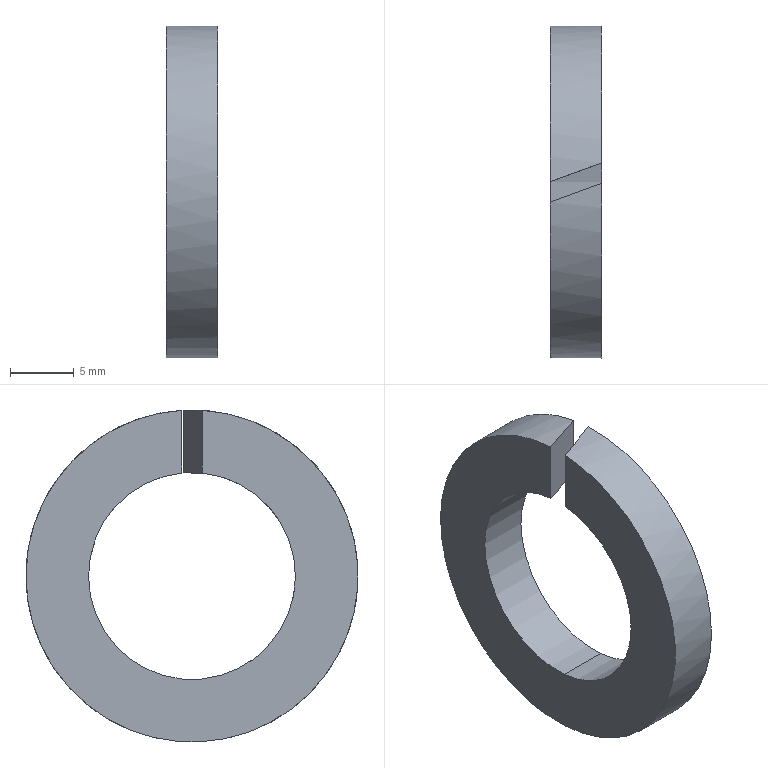Part | STEP file | KS B 1324 - No. 2 - 16 | 1 solid | 8 faces | box 4 x 26 x 26 mm | volume 1268 mm3 | cylinder 4 | plane 4 | commonest cylinder face diameters 16.2 x2 26 x2
STEP:
#1=CARTESIAN_POINT('',(0.,0.,0.));
#2=DIRECTION('',(0.,0.,1.));
#3=DIRECTION('',(1.,0.,0.));
#4=AXIS2_PLACEMENT_3D('',#1,#2,#3);
#5=CARTESIAN_POINT('',(4.,2.256,7.78));
#6=VERTEX_POINT('',#5);
#7=CARTESIAN_POINT('',(0.,0.8,8.06));
#8=VERTEX_POINT('',#7);
#9=CARTESIAN_POINT('',(4.,2.256,7.78));
#10=CARTESIAN_POINT('',(2.692,1.78,7.918));
#11=CARTESIAN_POINT('',(1.355,1.293,8.011));
#12=CARTESIAN_POINT('',(0.,0.8,8.06));
#13=(BOUNDED_CURVE()B_SPLINE_CURVE(3,(#9,#10,#11,#12),.UNSPECIFIED.,.F.,.F.)B_SPLINE_CURVE_WITH_KNOTS((4,4),(4.43,4.613),.PIECEWISE_BEZIER_KNOTS.)CURVE()GEOMETRIC_REPRESENTATION_ITEM()RATIONAL_B_SPLINE_CURVE((1.,0.9972,0.9972,1.))REPRESENTATION_ITEM(''));
#14=CARTESIAN_POINT('',(0.,0.,0.));
#15=DIRECTION('',(1.,0.,0.));
#16=DIRECTION('',(0.,-0.08987,-0.996));
#17=AXIS2_PLACEMENT_3D('',#14,#15,#16);
#18=CYLINDRICAL_SURFACE('',#17,8.1);
#19=CARTESIAN_POINT('',(2.949,4.));
#20=CARTESIAN_POINT('',(2.952,3.941));
#21=CARTESIAN_POINT('',(2.958,3.822));
#22=CARTESIAN_POINT('',(2.966,3.643));
#23=CARTESIAN_POINT('',(2.974,3.464));
#24=CARTESIAN_POINT('',(2.983,3.285));
#25=CARTESIAN_POINT('',(2.991,3.105));
#26=CARTESIAN_POINT('',(2.999,2.925));
#27=CARTESIAN_POINT('',(3.008,2.744));
#28=CARTESIAN_POINT('',(3.016,2.563));
#29=CARTESIAN_POINT('',(3.024,2.382));
#30=CARTESIAN_POINT('',(3.033,2.2));
#31=CARTESIAN_POINT('',(3.041,2.018));
#32=CARTESIAN_POINT('',(3.049,1.835));
#33=CARTESIAN_POINT('',(3.058,1.653));
#34=CARTESIAN_POINT('',(3.066,1.47));
#35=CARTESIAN_POINT('',(3.074,1.287));
#36=CARTESIAN_POINT('',(3.083,1.103));
#37=CARTESIAN_POINT('',(3.091,0.9199));
#38=CARTESIAN_POINT('',(3.099,0.7362));
#39=CARTESIAN_POINT('',(3.108,0.5524));
#40=CARTESIAN_POINT('',(3.116,0.3684));
#41=CARTESIAN_POINT('',(3.124,0.1842));
#42=CARTESIAN_POINT('',(3.13,0.06142));
#43=CARTESIAN_POINT('',(3.133,0.));
#44=B_SPLINE_CURVE_WITH_KNOTS('',3,(#19,#20,#21,#22,#23,#24,#25,#26,#27,#28,#29,#30,#31,#32,#33,#34,#35,#36,#37,#38,#39,#40,#41,#42,#43),.UNSPECIFIED.,.F.,.F.,(4,1,1,1,1,1,1,1,1,1,1,1,1,1,1,1,1,1,1,1,1,1,4),(4.43,4.438,4.447,4.455,4.463,4.472,4.48,4.488,4.497,4.505,4.513,4.522,4.53,4.538,4.547,4.555,4.563,4.572,4.58,4.588,4.597,4.605,4.613),.QUASI_UNIFORM_KNOTS.);
#45=(GEOMETRIC_REPRESENTATION_CONTEXT(2)PARAMETRIC_REPRESENTATION_CONTEXT()REPRESENTATION_CONTEXT('',''));
#46=DEFINITIONAL_REPRESENTATION('',(#44),#45);
#47=PCURVE('',#18,#46);
#48=CARTESIAN_POINT('',(0.,0.8,0.));
#49=DIRECTION('',(-0.342,0.9397,0.));
#50=DIRECTION('',(0.,0.,1.));
#51=AXIS2_PLACEMENT_3D('',#48,#49,#50);
#52=PLANE('',#51);
#53=CARTESIAN_POINT('',(7.78,4.257));
#54=CARTESIAN_POINT('',(7.918,2.865));
#55=CARTESIAN_POINT('',(8.011,1.442));
#56=CARTESIAN_POINT('',(8.06,0.));
#57=(BOUNDED_CURVE()B_SPLINE_CURVE(3,(#53,#54,#55,#56),.UNSPECIFIED.,.F.,.F.)B_SPLINE_CURVE_WITH_KNOTS((4,4),(4.43,4.613),.PIECEWISE_BEZIER_KNOTS.)CURVE()GEOMETRIC_REPRESENTATION_ITEM()RATIONAL_B_SPLINE_CURVE((1.,0.9972,0.9972,1.))REPRESENTATION_ITEM(''));
#58=(GEOMETRIC_REPRESENTATION_CONTEXT(2)PARAMETRIC_REPRESENTATION_CONTEXT()REPRESENTATION_CONTEXT('',''));
#59=DEFINITIONAL_REPRESENTATION('',(#57),#58);
#60=PCURVE('',#52,#59);
#61=SURFACE_CURVE('',#13,(#47,#60),.PCURVE_S1.);
#62=EDGE_CURVE('',#6,#8,#61,.T.);
#63=ORIENTED_EDGE('',*,*,#62,.F.);
#64=CARTESIAN_POINT('',(4.,-0.728,-8.067));
#65=VERTEX_POINT('',#64);
#66=CARTESIAN_POINT('',(4.,0.,0.));
#67=DIRECTION('',(-1.,0.,0.));
#68=DIRECTION('',(0.,-1.,0.));
#69=AXIS2_PLACEMENT_3D('',#66,#67,#68);
#70=CIRCLE('',#69,8.1);
#71=CARTESIAN_POINT('',(4.802,4.));
#72=DIRECTION('',(-1.,0.));
#73=VECTOR('',#72,1.);
#74=LINE('',#71,#73);
#75=(GEOMETRIC_REPRESENTATION_CONTEXT(2)PARAMETRIC_REPRESENTATION_CONTEXT()REPRESENTATION_CONTEXT('',''));
#76=DEFINITIONAL_REPRESENTATION('',(#74),#75);
#77=PCURVE('',#18,#76);
#78=CARTESIAN_POINT('',(4.,0.,0.));
#79=DIRECTION('',(-1.,0.,0.));
#80=DIRECTION('',(0.,0.,1.));
#81=AXIS2_PLACEMENT_3D('',#78,#79,#80);
#82=PLANE('',#81);
#83=CARTESIAN_POINT('',(0.,0.));
#84=DIRECTION('',(0.,-1.));
#85=AXIS2_PLACEMENT_2D('',#83,#84);
#86=CIRCLE('',#85,8.1);
#87=(GEOMETRIC_REPRESENTATION_CONTEXT(2)PARAMETRIC_REPRESENTATION_CONTEXT()REPRESENTATION_CONTEXT('',''));
#88=DEFINITIONAL_REPRESENTATION('',(#86),#87);
#89=PCURVE('',#82,#88);
#90=SURFACE_CURVE('',#70,(#77,#89),.PCURVE_S1.);
#91=EDGE_CURVE('',#6,#65,#90,.T.);
#92=ORIENTED_EDGE('',*,*,#91,.T.);
#93=CARTESIAN_POINT('',(0.,-0.728,-8.067));
#94=VERTEX_POINT('',#93);
#95=CARTESIAN_POINT('',(0.,-0.728,-8.067));
#96=DIRECTION('',(1.,0.,0.));
#97=VECTOR('',#96,1.);
#98=LINE('',#95,#97);
#99=CARTESIAN_POINT('',(0.,0.));
#100=DIRECTION('',(0.,1.));
#101=VECTOR('',#100,1.);
#102=LINE('',#99,#101);
#103=(GEOMETRIC_REPRESENTATION_CONTEXT(2)PARAMETRIC_REPRESENTATION_CONTEXT()REPRESENTATION_CONTEXT('',''));
#104=DEFINITIONAL_REPRESENTATION('',(#102),#103);
#105=PCURVE('',#18,#104);
#106=CARTESIAN_POINT('',(0.,0.,0.));
#107=DIRECTION('',(1.,0.,0.));
#108=DIRECTION('',(0.,-0.08987,-0.996));
#109=AXIS2_PLACEMENT_3D('',#106,#107,#108);
#110=CYLINDRICAL_SURFACE('',#109,8.1);
#111=CARTESIAN_POINT('',(6.283,0.));
#112=DIRECTION('',(0.,1.));
#113=VECTOR('',#112,1.);
#114=LINE('',#111,#113);
#115=(GEOMETRIC_REPRESENTATION_CONTEXT(2)PARAMETRIC_REPRESENTATION_CONTEXT()REPRESENTATION_CONTEXT('',''));
#116=DEFINITIONAL_REPRESENTATION('',(#114),#115);
#117=PCURVE('',#110,#116);
#118=SURFACE_CURVE('',#98,(#105,#117),.PCURVE_S1.);
#119=EDGE_CURVE('',#94,#65,#118,.T.);
#120=ORIENTED_EDGE('',*,*,#119,.F.);
#121=CARTESIAN_POINT('',(0.,0.,0.));
#122=DIRECTION('',(1.,0.,0.));
#123=DIRECTION('',(0.,-1.,0.));
#124=AXIS2_PLACEMENT_3D('',#121,#122,#123);
#125=CIRCLE('',#124,8.1);
#126=CARTESIAN_POINT('',(-1.481,0.));
#127=DIRECTION('',(1.,0.));
#128=VECTOR('',#127,1.);
#129=LINE('',#126,#128);
#130=(GEOMETRIC_REPRESENTATION_CONTEXT(2)PARAMETRIC_REPRESENTATION_CONTEXT()REPRESENTATION_CONTEXT('',''));
#131=DEFINITIONAL_REPRESENTATION('',(#129),#130);
#132=PCURVE('',#18,#131);
#133=CARTESIAN_POINT('',(0.,0.,0.));
#134=DIRECTION('',(-1.,0.,0.));
#135=DIRECTION('',(0.,0.,1.));
#136=AXIS2_PLACEMENT_3D('',#133,#134,#135);
#137=PLANE('',#136);
#138=CARTESIAN_POINT('',(0.,-8.1));
#139=CARTESIAN_POINT('',(-14.03,-8.1));
#140=CARTESIAN_POINT('',(-7.015,4.05));
#141=CARTESIAN_POINT('',(0.,16.2));
#142=CARTESIAN_POINT('',(7.015,4.05));
#143=CARTESIAN_POINT('',(14.03,-8.1));
#144=CARTESIAN_POINT('',(0.,-8.1));
#145=(BOUNDED_CURVE()B_SPLINE_CURVE(2,(#138,#139,#140,#141,#142,#143,#144),.UNSPECIFIED.,.T.,.F.)B_SPLINE_CURVE_WITH_KNOTS((1,2,2,2,2,1),(-2.094,0.,2.094,4.189,6.283,8.378),.UNSPECIFIED.)CURVE()GEOMETRIC_REPRESENTATION_ITEM()RATIONAL_B_SPLINE_CURVE((1.,0.5,1.,0.5,1.,0.5,1.))REPRESENTATION_ITEM(''));
#146=(GEOMETRIC_REPRESENTATION_CONTEXT(2)PARAMETRIC_REPRESENTATION_CONTEXT()REPRESENTATION_CONTEXT('',''));
#147=DEFINITIONAL_REPRESENTATION('',(#145),#146);
#148=PCURVE('',#137,#147);
#149=SURFACE_CURVE('',#125,(#132,#148),.PCURVE_S1.);
#150=EDGE_CURVE('',#94,#8,#149,.T.);
#151=ORIENTED_EDGE('',*,*,#150,.T.);
#152=EDGE_LOOP('',(#63,#92,#120,#151));
#153=FACE_BOUND('',#152,.F.);
#154=ADVANCED_FACE('',(#153),#18,.F.);
#155=CARTESIAN_POINT('',(0.,-0.728,-12.98));
#156=VERTEX_POINT('',#155);
#157=CARTESIAN_POINT('',(0.,-0.8,12.975));
#158=VERTEX_POINT('',#157);
#159=CARTESIAN_POINT('',(0.,0.,0.));
#160=DIRECTION('',(-1.,0.,0.));
#161=DIRECTION('',(0.,-1.,0.));
#162=AXIS2_PLACEMENT_3D('',#159,#160,#161);
#163=CIRCLE('',#162,13.);
#164=CARTESIAN_POINT('',(0.,0.,0.));
#165=DIRECTION('',(1.,0.,0.));
#166=DIRECTION('',(0.,-0.056,-0.9984));
#167=AXIS2_PLACEMENT_3D('',#164,#165,#166);
#168=CYLINDRICAL_SURFACE('',#167,13.);
#169=CARTESIAN_POINT('',(11.052,0.));
#170=DIRECTION('',(-1.,0.));
#171=VECTOR('',#170,1.);
#172=LINE('',#169,#171);
#173=(GEOMETRIC_REPRESENTATION_CONTEXT(2)PARAMETRIC_REPRESENTATION_CONTEXT()REPRESENTATION_CONTEXT('',''));
#174=DEFINITIONAL_REPRESENTATION('',(#172),#173);
#175=PCURVE('',#168,#174);
#176=CARTESIAN_POINT('',(0.,0.));
#177=DIRECTION('',(0.,-1.));
#178=AXIS2_PLACEMENT_2D('',#176,#177);
#179=CIRCLE('',#178,13.);
#180=(GEOMETRIC_REPRESENTATION_CONTEXT(2)PARAMETRIC_REPRESENTATION_CONTEXT()REPRESENTATION_CONTEXT('',''));
#181=DEFINITIONAL_REPRESENTATION('',(#179),#180);
#182=PCURVE('',#137,#181);
#183=SURFACE_CURVE('',#163,(#175,#182),.PCURVE_S1.);
#184=EDGE_CURVE('',#156,#158,#183,.T.);
#185=ORIENTED_EDGE('',*,*,#184,.F.);
#186=CARTESIAN_POINT('',(4.,-0.728,-12.98));
#187=VERTEX_POINT('',#186);
#188=CARTESIAN_POINT('',(0.,-0.728,-12.98));
#189=DIRECTION('',(1.,0.,0.));
#190=VECTOR('',#189,1.);
#191=LINE('',#188,#190);
#192=CARTESIAN_POINT('',(6.283,0.));
#193=DIRECTION('',(0.,1.));
#194=VECTOR('',#193,1.);
#195=LINE('',#192,#194);
#196=(GEOMETRIC_REPRESENTATION_CONTEXT(2)PARAMETRIC_REPRESENTATION_CONTEXT()REPRESENTATION_CONTEXT('',''));
#197=DEFINITIONAL_REPRESENTATION('',(#195),#196);
#198=PCURVE('',#168,#197);
#199=CARTESIAN_POINT('',(0.,0.,0.));
#200=DIRECTION('',(1.,0.,0.));
#201=DIRECTION('',(0.,-0.056,-0.9984));
#202=AXIS2_PLACEMENT_3D('',#199,#200,#201);
#203=CYLINDRICAL_SURFACE('',#202,13.);
#204=CARTESIAN_POINT('',(0.,0.));
#205=DIRECTION('',(0.,1.));
#206=VECTOR('',#205,1.);
#207=LINE('',#204,#206);
#208=(GEOMETRIC_REPRESENTATION_CONTEXT(2)PARAMETRIC_REPRESENTATION_CONTEXT()REPRESENTATION_CONTEXT('',''));
#209=DEFINITIONAL_REPRESENTATION('',(#207),#208);
#210=PCURVE('',#203,#209);
#211=SURFACE_CURVE('',#191,(#198,#210),.PCURVE_S1.);
#212=EDGE_CURVE('',#156,#187,#211,.T.);
#213=ORIENTED_EDGE('',*,*,#212,.T.);
#214=CARTESIAN_POINT('',(4.,0.6559,12.983));
#215=VERTEX_POINT('',#214);
#216=CARTESIAN_POINT('',(4.,0.,0.));
#217=DIRECTION('',(-1.,0.,0.));
#218=DIRECTION('',(0.,-1.,0.));
#219=AXIS2_PLACEMENT_3D('',#216,#217,#218);
#220=CIRCLE('',#219,13.);
#221=CARTESIAN_POINT('',(11.052,4.));
#222=DIRECTION('',(-1.,0.));
#223=VECTOR('',#222,1.);
#224=LINE('',#221,#223);
#225=(GEOMETRIC_REPRESENTATION_CONTEXT(2)PARAMETRIC_REPRESENTATION_CONTEXT()REPRESENTATION_CONTEXT('',''));
#226=DEFINITIONAL_REPRESENTATION('',(#224),#225);
#227=PCURVE('',#168,#226);
#228=CARTESIAN_POINT('',(0.,0.));
#229=DIRECTION('',(0.,-1.));
#230=AXIS2_PLACEMENT_2D('',#228,#229);
#231=CIRCLE('',#230,13.);
#232=(GEOMETRIC_REPRESENTATION_CONTEXT(2)PARAMETRIC_REPRESENTATION_CONTEXT()REPRESENTATION_CONTEXT('',''));
#233=DEFINITIONAL_REPRESENTATION('',(#231),#232);
#234=PCURVE('',#82,#233);
#235=SURFACE_CURVE('',#220,(#227,#234),.PCURVE_S1.);
#236=EDGE_CURVE('',#187,#215,#235,.T.);
#237=ORIENTED_EDGE('',*,*,#236,.T.);
#238=CARTESIAN_POINT('',(4.,0.6559,12.983));
#239=CARTESIAN_POINT('',(2.667,0.1707,13.008));
#240=CARTESIAN_POINT('',(1.332,-0.3151,13.005));
#241=CARTESIAN_POINT('',(0.,-0.8,12.975));
#242=(BOUNDED_CURVE()B_SPLINE_CURVE(3,(#238,#239,#240,#241),.UNSPECIFIED.,.F.,.F.)B_SPLINE_CURVE_WITH_KNOTS((4,4),(4.662,4.774),.PIECEWISE_BEZIER_KNOTS.)CURVE()GEOMETRIC_REPRESENTATION_ITEM()RATIONAL_B_SPLINE_CURVE((1.,0.999,0.999,1.))REPRESENTATION_ITEM(''));
#243=CARTESIAN_POINT('',(3.147,4.));
#244=CARTESIAN_POINT('',(3.149,3.939));
#245=CARTESIAN_POINT('',(3.152,3.818));
#246=CARTESIAN_POINT('',(3.157,3.637));
#247=CARTESIAN_POINT('',(3.162,3.455));
#248=CARTESIAN_POINT('',(3.168,3.273));
#249=CARTESIAN_POINT('',(3.173,3.091));
#250=CARTESIAN_POINT('',(3.178,2.909));
#251=CARTESIAN_POINT('',(3.183,2.728));
#252=CARTESIAN_POINT('',(3.188,2.546));
#253=CARTESIAN_POINT('',(3.193,2.364));
#254=CARTESIAN_POINT('',(3.198,2.182));
#255=CARTESIAN_POINT('',(3.203,2.));
#256=CARTESIAN_POINT('',(3.208,1.818));
#257=CARTESIAN_POINT('',(3.213,1.636));
#258=CARTESIAN_POINT('',(3.218,1.454));
#259=CARTESIAN_POINT('',(3.224,1.272));
#260=CARTESIAN_POINT('',(3.229,1.09));
#261=CARTESIAN_POINT('',(3.234,0.9083));
#262=CARTESIAN_POINT('',(3.239,0.7265));
#263=CARTESIAN_POINT('',(3.244,0.5448));
#264=CARTESIAN_POINT('',(3.249,0.3631));
#265=CARTESIAN_POINT('',(3.254,0.1815));
#266=CARTESIAN_POINT('',(3.257,0.06049));
#267=CARTESIAN_POINT('',(3.259,0.));
#268=B_SPLINE_CURVE_WITH_KNOTS('',3,(#243,#244,#245,#246,#247,#248,#249,#250,#251,#252,#253,#254,#255,#256,#257,#258,#259,#260,#261,#262,#263,#264,#265,#266,#267),.UNSPECIFIED.,.F.,.F.,(4,1,1,1,1,1,1,1,1,1,1,1,1,1,1,1,1,1,1,1,1,1,4),(4.662,4.667,4.672,4.677,4.682,4.687,4.692,4.698,4.703,4.708,4.713,4.718,4.723,4.728,4.733,4.738,4.743,4.749,4.754,4.759,4.764,4.769,4.774),.QUASI_UNIFORM_KNOTS.);
#269=(GEOMETRIC_REPRESENTATION_CONTEXT(2)PARAMETRIC_REPRESENTATION_CONTEXT()REPRESENTATION_CONTEXT('',''));
#270=DEFINITIONAL_REPRESENTATION('',(#268),#269);
#271=PCURVE('',#168,#270);
#272=CARTESIAN_POINT('',(4.,0.6559,0.));
#273=DIRECTION('',(0.342,-0.9397,0.));
#274=DIRECTION('',(0.,0.,-1.));
#275=AXIS2_PLACEMENT_3D('',#272,#273,#274);
#276=PLANE('',#275);
#277=CARTESIAN_POINT('',(-12.983,0.));
#278=CARTESIAN_POINT('',(-13.008,-1.419));
#279=CARTESIAN_POINT('',(-13.005,-2.839));
#280=CARTESIAN_POINT('',(-12.975,-4.257));
#281=(BOUNDED_CURVE()B_SPLINE_CURVE(3,(#277,#278,#279,#280),.UNSPECIFIED.,.F.,.F.)B_SPLINE_CURVE_WITH_KNOTS((4,4),(4.662,4.774),.PIECEWISE_BEZIER_KNOTS.)CURVE()GEOMETRIC_REPRESENTATION_ITEM()RATIONAL_B_SPLINE_CURVE((1.,0.999,0.999,1.))REPRESENTATION_ITEM(''));
#282=(GEOMETRIC_REPRESENTATION_CONTEXT(2)PARAMETRIC_REPRESENTATION_CONTEXT()REPRESENTATION_CONTEXT('',''));
#283=DEFINITIONAL_REPRESENTATION('',(#281),#282);
#284=PCURVE('',#276,#283);
#285=SURFACE_CURVE('',#242,(#271,#284),.PCURVE_S1.);
#286=EDGE_CURVE('',#215,#158,#285,.T.);
#287=ORIENTED_EDGE('',*,*,#286,.T.);
#288=EDGE_LOOP('',(#185,#213,#237,#287));
#289=FACE_BOUND('',#288,.T.);
#290=ADVANCED_FACE('',(#289),#168,.T.);
#291=CARTESIAN_POINT('',(0.,-0.8,8.06));
#292=VERTEX_POINT('',#291);
#293=CARTESIAN_POINT('',(0.,-0.8,0.));
#294=DIRECTION('',(0.,0.,-1.));
#295=VECTOR('',#294,1.);
#296=LINE('',#293,#295);
#297=CARTESIAN_POINT('',(0.,-0.8));
#298=DIRECTION('',(-1.,0.));
#299=VECTOR('',#298,1.);
#300=LINE('',#297,#299);
#301=(GEOMETRIC_REPRESENTATION_CONTEXT(2)PARAMETRIC_REPRESENTATION_CONTEXT()REPRESENTATION_CONTEXT('',''));
#302=DEFINITIONAL_REPRESENTATION('',(#300),#301);
#303=PCURVE('',#137,#302);
#304=CARTESIAN_POINT('',(0.,-4.257));
#305=DIRECTION('',(1.,0.));
#306=VECTOR('',#305,1.);
#307=LINE('',#304,#306);
#308=(GEOMETRIC_REPRESENTATION_CONTEXT(2)PARAMETRIC_REPRESENTATION_CONTEXT()REPRESENTATION_CONTEXT('',''));
#309=DEFINITIONAL_REPRESENTATION('',(#307),#308);
#310=PCURVE('',#276,#309);
#311=SURFACE_CURVE('',#296,(#303,#310),.PCURVE_S1.);
#312=EDGE_CURVE('',#158,#292,#311,.T.);
#313=ORIENTED_EDGE('',*,*,#312,.T.);
#314=CARTESIAN_POINT('',(0.,0.,0.));
#315=DIRECTION('',(1.,0.,0.));
#316=DIRECTION('',(0.,-1.,0.));
#317=AXIS2_PLACEMENT_3D('',#314,#315,#316);
#318=CIRCLE('',#317,8.1);
#319=CARTESIAN_POINT('',(0.,-8.1));
#320=CARTESIAN_POINT('',(-14.03,-8.1));
#321=CARTESIAN_POINT('',(-7.015,4.05));
#322=CARTESIAN_POINT('',(0.,16.2));
#323=CARTESIAN_POINT('',(7.015,4.05));
#324=CARTESIAN_POINT('',(14.03,-8.1));
#325=CARTESIAN_POINT('',(0.,-8.1));
#326=(BOUNDED_CURVE()B_SPLINE_CURVE(2,(#319,#320,#321,#322,#323,#324,#325),.UNSPECIFIED.,.T.,.F.)B_SPLINE_CURVE_WITH_KNOTS((1,2,2,2,2,1),(-2.094,0.,2.094,4.189,6.283,8.378),.UNSPECIFIED.)CURVE()GEOMETRIC_REPRESENTATION_ITEM()RATIONAL_B_SPLINE_CURVE((1.,0.5,1.,0.5,1.,0.5,1.))REPRESENTATION_ITEM(''));
#327=(GEOMETRIC_REPRESENTATION_CONTEXT(2)PARAMETRIC_REPRESENTATION_CONTEXT()REPRESENTATION_CONTEXT('',''));
#328=DEFINITIONAL_REPRESENTATION('',(#326),#327);
#329=PCURVE('',#137,#328);
#330=CARTESIAN_POINT('',(-1.481,0.));
#331=DIRECTION('',(1.,0.));
#332=VECTOR('',#331,1.);
#333=LINE('',#330,#332);
#334=(GEOMETRIC_REPRESENTATION_CONTEXT(2)PARAMETRIC_REPRESENTATION_CONTEXT()REPRESENTATION_CONTEXT('',''));
#335=DEFINITIONAL_REPRESENTATION('',(#333),#334);
#336=PCURVE('',#110,#335);
#337=SURFACE_CURVE('',#318,(#329,#336),.PCURVE_S1.);
#338=EDGE_CURVE('',#292,#94,#337,.T.);
#339=ORIENTED_EDGE('',*,*,#338,.T.);
#340=ORIENTED_EDGE('',*,*,#150,.T.);
#341=CARTESIAN_POINT('',(0.,0.8,12.975));
#342=VERTEX_POINT('',#341);
#343=CARTESIAN_POINT('',(0.,0.8,0.));
#344=DIRECTION('',(0.,0.,1.));
#345=VECTOR('',#344,1.);
#346=LINE('',#343,#345);
#347=CARTESIAN_POINT('',(0.,0.8));
#348=DIRECTION('',(1.,0.));
#349=VECTOR('',#348,1.);
#350=LINE('',#347,#349);
#351=(GEOMETRIC_REPRESENTATION_CONTEXT(2)PARAMETRIC_REPRESENTATION_CONTEXT()REPRESENTATION_CONTEXT('',''));
#352=DEFINITIONAL_REPRESENTATION('',(#350),#351);
#353=PCURVE('',#137,#352);
#354=CARTESIAN_POINT('',(0.,0.));
#355=DIRECTION('',(1.,0.));
#356=VECTOR('',#355,1.);
#357=LINE('',#354,#356);
#358=(GEOMETRIC_REPRESENTATION_CONTEXT(2)PARAMETRIC_REPRESENTATION_CONTEXT()REPRESENTATION_CONTEXT('',''));
#359=DEFINITIONAL_REPRESENTATION('',(#357),#358);
#360=PCURVE('',#52,#359);
#361=SURFACE_CURVE('',#346,(#353,#360),.PCURVE_S1.);
#362=EDGE_CURVE('',#8,#342,#361,.T.);
#363=ORIENTED_EDGE('',*,*,#362,.T.);
#364=CARTESIAN_POINT('',(0.,0.,0.));
#365=DIRECTION('',(-1.,0.,0.));
#366=DIRECTION('',(0.,-1.,0.));
#367=AXIS2_PLACEMENT_3D('',#364,#365,#366);
#368=CIRCLE('',#367,13.);
#369=CARTESIAN_POINT('',(0.,0.));
#370=DIRECTION('',(0.,-1.));
#371=AXIS2_PLACEMENT_2D('',#369,#370);
#372=CIRCLE('',#371,13.);
#373=(GEOMETRIC_REPRESENTATION_CONTEXT(2)PARAMETRIC_REPRESENTATION_CONTEXT()REPRESENTATION_CONTEXT('',''));
#374=DEFINITIONAL_REPRESENTATION('',(#372),#373);
#375=PCURVE('',#137,#374);
#376=CARTESIAN_POINT('',(4.768,0.));
#377=DIRECTION('',(-1.,0.));
#378=VECTOR('',#377,1.);
#379=LINE('',#376,#378);
#380=(GEOMETRIC_REPRESENTATION_CONTEXT(2)PARAMETRIC_REPRESENTATION_CONTEXT()REPRESENTATION_CONTEXT('',''));
#381=DEFINITIONAL_REPRESENTATION('',(#379),#380);
#382=PCURVE('',#203,#381);
#383=SURFACE_CURVE('',#368,(#375,#382),.PCURVE_S1.);
#384=EDGE_CURVE('',#342,#156,#383,.T.);
#385=ORIENTED_EDGE('',*,*,#384,.T.);
#386=ORIENTED_EDGE('',*,*,#184,.T.);
#387=EDGE_LOOP('',(#313,#339,#340,#363,#385,#386));
#388=FACE_BOUND('',#387,.T.);
#389=ADVANCED_FACE('',(#388),#137,.T.);
#390=ORIENTED_EDGE('',*,*,#212,.F.);
#391=ORIENTED_EDGE('',*,*,#384,.F.);
#392=CARTESIAN_POINT('',(4.,2.256,12.803));
#393=VERTEX_POINT('',#392);
#394=CARTESIAN_POINT('',(0.,0.8,12.975));
#395=CARTESIAN_POINT('',(1.342,1.288,12.945));
#396=CARTESIAN_POINT('',(2.676,1.774,12.888));
#397=CARTESIAN_POINT('',(4.,2.256,12.803));
#398=(BOUNDED_CURVE()B_SPLINE_CURVE(3,(#394,#395,#396,#397),.UNSPECIFIED.,.F.,.F.)B_SPLINE_CURVE_WITH_KNOTS((4,4),(1.632,1.745),.PIECEWISE_BEZIER_KNOTS.)CURVE()GEOMETRIC_REPRESENTATION_ITEM()RATIONAL_B_SPLINE_CURVE((1.,0.9989,0.9989,1.))REPRESENTATION_ITEM(''));
#399=CARTESIAN_POINT('',(3.136,0.));
#400=CARTESIAN_POINT('',(3.134,0.06091));
#401=CARTESIAN_POINT('',(3.131,0.1827));
#402=CARTESIAN_POINT('',(3.126,0.3654));
#403=CARTESIAN_POINT('',(3.121,0.5481));
#404=CARTESIAN_POINT('',(3.116,0.7307));
#405=CARTESIAN_POINT('',(3.11,0.9132));
#406=CARTESIAN_POINT('',(3.105,1.096));
#407=CARTESIAN_POINT('',(3.1,1.278));
#408=CARTESIAN_POINT('',(3.095,1.46));
#409=CARTESIAN_POINT('',(3.09,1.643));
#410=CARTESIAN_POINT('',(3.085,1.825));
#411=CARTESIAN_POINT('',(3.08,2.007));
#412=CARTESIAN_POINT('',(3.074,2.189));
#413=CARTESIAN_POINT('',(3.069,2.37));
#414=CARTESIAN_POINT('',(3.064,2.552));
#415=CARTESIAN_POINT('',(3.059,2.734));
#416=CARTESIAN_POINT('',(3.054,2.915));
#417=CARTESIAN_POINT('',(3.049,3.096));
#418=CARTESIAN_POINT('',(3.044,3.277));
#419=CARTESIAN_POINT('',(3.039,3.458));
#420=CARTESIAN_POINT('',(3.033,3.639));
#421=CARTESIAN_POINT('',(3.028,3.82));
#422=CARTESIAN_POINT('',(3.025,3.94));
#423=CARTESIAN_POINT('',(3.023,4.));
#424=B_SPLINE_CURVE_WITH_KNOTS('',3,(#399,#400,#401,#402,#403,#404,#405,#406,#407,#408,#409,#410,#411,#412,#413,#414,#415,#416,#417,#418,#419,#420,#421,#422,#423),.UNSPECIFIED.,.F.,.F.,(4,1,1,1,1,1,1,1,1,1,1,1,1,1,1,1,1,1,1,1,1,1,4),(1.632,1.638,1.643,1.648,1.653,1.658,1.663,1.668,1.673,1.679,1.684,1.689,1.694,1.699,1.704,1.709,1.714,1.72,1.725,1.73,1.735,1.74,1.745),.QUASI_UNIFORM_KNOTS.);
#425=(GEOMETRIC_REPRESENTATION_CONTEXT(2)PARAMETRIC_REPRESENTATION_CONTEXT()REPRESENTATION_CONTEXT('',''));
#426=DEFINITIONAL_REPRESENTATION('',(#424),#425);
#427=PCURVE('',#203,#426);
#428=CARTESIAN_POINT('',(12.975,0.));
#429=CARTESIAN_POINT('',(12.945,1.428));
#430=CARTESIAN_POINT('',(12.888,2.848));
#431=CARTESIAN_POINT('',(12.803,4.257));
#432=(BOUNDED_CURVE()B_SPLINE_CURVE(3,(#428,#429,#430,#431),.UNSPECIFIED.,.F.,.F.)B_SPLINE_CURVE_WITH_KNOTS((4,4),(1.632,1.745),.PIECEWISE_BEZIER_KNOTS.)CURVE()GEOMETRIC_REPRESENTATION_ITEM()RATIONAL_B_SPLINE_CURVE((1.,0.9989,0.9989,1.))REPRESENTATION_ITEM(''));
#433=(GEOMETRIC_REPRESENTATION_CONTEXT(2)PARAMETRIC_REPRESENTATION_CONTEXT()REPRESENTATION_CONTEXT('',''));
#434=DEFINITIONAL_REPRESENTATION('',(#432),#433);
#435=PCURVE('',#52,#434);
#436=SURFACE_CURVE('',#398,(#427,#435),.PCURVE_S1.);
#437=EDGE_CURVE('',#342,#393,#436,.T.);
#438=ORIENTED_EDGE('',*,*,#437,.T.);
#439=CARTESIAN_POINT('',(4.,0.,0.));
#440=DIRECTION('',(-1.,0.,0.));
#441=DIRECTION('',(0.,-1.,0.));
#442=AXIS2_PLACEMENT_3D('',#439,#440,#441);
#443=CIRCLE('',#442,13.);
#444=CARTESIAN_POINT('',(4.768,4.));
#445=DIRECTION('',(-1.,0.));
#446=VECTOR('',#445,1.);
#447=LINE('',#444,#446);
#448=(GEOMETRIC_REPRESENTATION_CONTEXT(2)PARAMETRIC_REPRESENTATION_CONTEXT()REPRESENTATION_CONTEXT('',''));
#449=DEFINITIONAL_REPRESENTATION('',(#447),#448);
#450=PCURVE('',#203,#449);
#451=CARTESIAN_POINT('',(0.,0.));
#452=DIRECTION('',(0.,-1.));
#453=AXIS2_PLACEMENT_2D('',#451,#452);
#454=CIRCLE('',#453,13.);
#455=(GEOMETRIC_REPRESENTATION_CONTEXT(2)PARAMETRIC_REPRESENTATION_CONTEXT()REPRESENTATION_CONTEXT('',''));
#456=DEFINITIONAL_REPRESENTATION('',(#454),#455);
#457=PCURVE('',#82,#456);
#458=SURFACE_CURVE('',#443,(#450,#457),.PCURVE_S1.);
#459=EDGE_CURVE('',#393,#187,#458,.T.);
#460=ORIENTED_EDGE('',*,*,#459,.T.);
#461=EDGE_LOOP('',(#390,#391,#438,#460));
#462=FACE_BOUND('',#461,.T.);
#463=ADVANCED_FACE('',(#462),#203,.T.);
#464=CARTESIAN_POINT('',(4.,0.6559,8.073));
#465=VERTEX_POINT('',#464);
#466=CARTESIAN_POINT('',(4.,0.,0.));
#467=DIRECTION('',(-1.,0.,0.));
#468=DIRECTION('',(0.,-1.,0.));
#469=AXIS2_PLACEMENT_3D('',#466,#467,#468);
#470=CIRCLE('',#469,8.1);
#471=CARTESIAN_POINT('',(11.086,4.));
#472=DIRECTION('',(-1.,0.));
#473=VECTOR('',#472,1.);
#474=LINE('',#471,#473);
#475=(GEOMETRIC_REPRESENTATION_CONTEXT(2)PARAMETRIC_REPRESENTATION_CONTEXT()REPRESENTATION_CONTEXT('',''));
#476=DEFINITIONAL_REPRESENTATION('',(#474),#475);
#477=PCURVE('',#110,#476);
#478=CARTESIAN_POINT('',(0.,0.));
#479=DIRECTION('',(0.,-1.));
#480=AXIS2_PLACEMENT_2D('',#478,#479);
#481=CIRCLE('',#480,8.1);
#482=(GEOMETRIC_REPRESENTATION_CONTEXT(2)PARAMETRIC_REPRESENTATION_CONTEXT()REPRESENTATION_CONTEXT('',''));
#483=DEFINITIONAL_REPRESENTATION('',(#481),#482);
#484=PCURVE('',#82,#483);
#485=SURFACE_CURVE('',#470,(#477,#484),.PCURVE_S1.);
#486=EDGE_CURVE('',#65,#465,#485,.T.);
#487=ORIENTED_EDGE('',*,*,#486,.T.);
#488=CARTESIAN_POINT('',(0.,-0.8,8.06));
#489=CARTESIAN_POINT('',(1.33,-0.3158,8.108));
#490=CARTESIAN_POINT('',(2.667,0.1709,8.113));
#491=CARTESIAN_POINT('',(4.,0.6559,8.073));
#492=(BOUNDED_CURVE()B_SPLINE_CURVE(3,(#488,#489,#490,#491),.UNSPECIFIED.,.F.,.F.)B_SPLINE_CURVE_WITH_KNOTS((4,4),(1.472,1.652),.PIECEWISE_BEZIER_KNOTS.)CURVE()GEOMETRIC_REPRESENTATION_ITEM()RATIONAL_B_SPLINE_CURVE((1.,0.9973,0.9973,1.))REPRESENTATION_ITEM(''));
#493=CARTESIAN_POINT('',(3.331,0.));
#494=CARTESIAN_POINT('',(3.328,0.06031));
#495=CARTESIAN_POINT('',(3.322,0.181));
#496=CARTESIAN_POINT('',(3.314,0.3622));
#497=CARTESIAN_POINT('',(3.306,0.5437));
#498=CARTESIAN_POINT('',(3.298,0.7252));
#499=CARTESIAN_POINT('',(3.29,0.907));
#500=CARTESIAN_POINT('',(3.281,1.089));
#501=CARTESIAN_POINT('',(3.273,1.271));
#502=CARTESIAN_POINT('',(3.265,1.453));
#503=CARTESIAN_POINT('',(3.257,1.635));
#504=CARTESIAN_POINT('',(3.249,1.817));
#505=CARTESIAN_POINT('',(3.241,1.999));
#506=CARTESIAN_POINT('',(3.232,2.181));
#507=CARTESIAN_POINT('',(3.224,2.364));
#508=CARTESIAN_POINT('',(3.216,2.546));
#509=CARTESIAN_POINT('',(3.208,2.728));
#510=CARTESIAN_POINT('',(3.2,2.91));
#511=CARTESIAN_POINT('',(3.191,3.092));
#512=CARTESIAN_POINT('',(3.183,3.274));
#513=CARTESIAN_POINT('',(3.175,3.456));
#514=CARTESIAN_POINT('',(3.167,3.637));
#515=CARTESIAN_POINT('',(3.159,3.819));
#516=CARTESIAN_POINT('',(3.153,3.94));
#517=CARTESIAN_POINT('',(3.151,4.));
#518=B_SPLINE_CURVE_WITH_KNOTS('',3,(#493,#494,#495,#496,#497,#498,#499,#500,#501,#502,#503,#504,#505,#506,#507,#508,#509,#510,#511,#512,#513,#514,#515,#516,#517),.UNSPECIFIED.,.F.,.F.,(4,1,1,1,1,1,1,1,1,1,1,1,1,1,1,1,1,1,1,1,1,1,4),(1.472,1.48,1.488,1.496,1.505,1.513,1.521,1.529,1.537,1.546,1.554,1.562,1.57,1.578,1.586,1.595,1.603,1.611,1.619,1.627,1.635,1.644,1.652),.QUASI_UNIFORM_KNOTS.);
#519=(GEOMETRIC_REPRESENTATION_CONTEXT(2)PARAMETRIC_REPRESENTATION_CONTEXT()REPRESENTATION_CONTEXT('',''));
#520=DEFINITIONAL_REPRESENTATION('',(#518),#519);
#521=PCURVE('',#110,#520);
#522=CARTESIAN_POINT('',(-8.06,-4.257));
#523=CARTESIAN_POINT('',(-8.108,-2.841));
#524=CARTESIAN_POINT('',(-8.113,-1.418));
#525=CARTESIAN_POINT('',(-8.073,0.));
#526=(BOUNDED_CURVE()B_SPLINE_CURVE(3,(#522,#523,#524,#525),.UNSPECIFIED.,.F.,.F.)B_SPLINE_CURVE_WITH_KNOTS((4,4),(1.472,1.652),.PIECEWISE_BEZIER_KNOTS.)CURVE()GEOMETRIC_REPRESENTATION_ITEM()RATIONAL_B_SPLINE_CURVE((1.,0.9973,0.9973,1.))REPRESENTATION_ITEM(''));
#527=(GEOMETRIC_REPRESENTATION_CONTEXT(2)PARAMETRIC_REPRESENTATION_CONTEXT()REPRESENTATION_CONTEXT('',''));
#528=DEFINITIONAL_REPRESENTATION('',(#526),#527);
#529=PCURVE('',#276,#528);
#530=SURFACE_CURVE('',#492,(#521,#529),.PCURVE_S1.);
#531=EDGE_CURVE('',#292,#465,#530,.T.);
#532=ORIENTED_EDGE('',*,*,#531,.F.);
#533=ORIENTED_EDGE('',*,*,#338,.T.);
#534=ORIENTED_EDGE('',*,*,#119,.T.);
#535=EDGE_LOOP('',(#487,#532,#533,#534));
#536=FACE_BOUND('',#535,.F.);
#537=ADVANCED_FACE('',(#536),#110,.F.);
#538=CARTESIAN_POINT('',(4.,0.6559,0.));
#539=DIRECTION('',(0.,0.,1.));
#540=VECTOR('',#539,1.);
#541=LINE('',#538,#540);
#542=CARTESIAN_POINT('',(0.,0.6559));
#543=DIRECTION('',(1.,0.));
#544=VECTOR('',#543,1.);
#545=LINE('',#542,#544);
#546=(GEOMETRIC_REPRESENTATION_CONTEXT(2)PARAMETRIC_REPRESENTATION_CONTEXT()REPRESENTATION_CONTEXT('',''));
#547=DEFINITIONAL_REPRESENTATION('',(#545),#546);
#548=PCURVE('',#82,#547);
#549=CARTESIAN_POINT('',(0.,0.));
#550=DIRECTION('',(-1.,0.));
#551=VECTOR('',#550,1.);
#552=LINE('',#549,#551);
#553=(GEOMETRIC_REPRESENTATION_CONTEXT(2)PARAMETRIC_REPRESENTATION_CONTEXT()REPRESENTATION_CONTEXT('',''));
#554=DEFINITIONAL_REPRESENTATION('',(#552),#553);
#555=PCURVE('',#276,#554);
#556=SURFACE_CURVE('',#541,(#548,#555),.PCURVE_S1.);
#557=EDGE_CURVE('',#465,#215,#556,.T.);
#558=ORIENTED_EDGE('',*,*,#557,.T.);
#559=ORIENTED_EDGE('',*,*,#236,.F.);
#560=ORIENTED_EDGE('',*,*,#459,.F.);
#561=CARTESIAN_POINT('',(4.,2.256,0.));
#562=DIRECTION('',(0.,0.,-1.));
#563=VECTOR('',#562,1.);
#564=LINE('',#561,#563);
#565=CARTESIAN_POINT('',(0.,2.256));
#566=DIRECTION('',(-1.,0.));
#567=VECTOR('',#566,1.);
#568=LINE('',#565,#567);
#569=(GEOMETRIC_REPRESENTATION_CONTEXT(2)PARAMETRIC_REPRESENTATION_CONTEXT()REPRESENTATION_CONTEXT('',''));
#570=DEFINITIONAL_REPRESENTATION('',(#568),#569);
#571=PCURVE('',#82,#570);
#572=CARTESIAN_POINT('',(0.,4.257));
#573=DIRECTION('',(-1.,0.));
#574=VECTOR('',#573,1.);
#575=LINE('',#572,#574);
#576=(GEOMETRIC_REPRESENTATION_CONTEXT(2)PARAMETRIC_REPRESENTATION_CONTEXT()REPRESENTATION_CONTEXT('',''));
#577=DEFINITIONAL_REPRESENTATION('',(#575),#576);
#578=PCURVE('',#52,#577);
#579=SURFACE_CURVE('',#564,(#571,#578),.PCURVE_S1.);
#580=EDGE_CURVE('',#393,#6,#579,.T.);
#581=ORIENTED_EDGE('',*,*,#580,.T.);
#582=ORIENTED_EDGE('',*,*,#91,.T.);
#583=ORIENTED_EDGE('',*,*,#486,.T.);
#584=EDGE_LOOP('',(#558,#559,#560,#581,#582,#583));
#585=FACE_BOUND('',#584,.T.);
#586=ADVANCED_FACE('',(#585),#82,.F.);
#587=ORIENTED_EDGE('',*,*,#531,.F.);
#588=ORIENTED_EDGE('',*,*,#312,.F.);
#589=ORIENTED_EDGE('',*,*,#286,.F.);
#590=ORIENTED_EDGE('',*,*,#557,.F.);
#591=EDGE_LOOP('',(#587,#588,#589,#590));
#592=FACE_BOUND('',#591,.T.);
#593=ADVANCED_FACE('',(#592),#276,.F.);
#594=ORIENTED_EDGE('',*,*,#62,.F.);
#595=ORIENTED_EDGE('',*,*,#580,.F.);
#596=ORIENTED_EDGE('',*,*,#437,.F.);
#597=ORIENTED_EDGE('',*,*,#362,.F.);
#598=EDGE_LOOP('',(#594,#595,#596,#597));
#599=FACE_BOUND('',#598,.T.);
#600=ADVANCED_FACE('',(#599),#52,.F.);
#601=CLOSED_SHELL('',(#154,#290,#389,#463,#537,#586,#593,#600));
#602=MANIFOLD_SOLID_BREP('',#601);
#603=(LENGTH_UNIT()NAMED_UNIT(*)SI_UNIT(.MILLI.,.METRE.));
#604=UNCERTAINTY_MEASURE_WITH_UNIT(LENGTH_MEASURE(0.0000001),#603,'','');
#605=(NAMED_UNIT(*)PLANE_ANGLE_UNIT()SI_UNIT($,.RADIAN.));
#606=(NAMED_UNIT(*)SI_UNIT($,.STERADIAN.)SOLID_ANGLE_UNIT());
#607=(GEOMETRIC_REPRESENTATION_CONTEXT(3)GLOBAL_UNCERTAINTY_ASSIGNED_CONTEXT((#604))GLOBAL_UNIT_ASSIGNED_CONTEXT((#603,#605,#606))REPRESENTATION_CONTEXT('',''));
#608=ADVANCED_BREP_SHAPE_REPRESENTATION('',(#4,#602),#607);